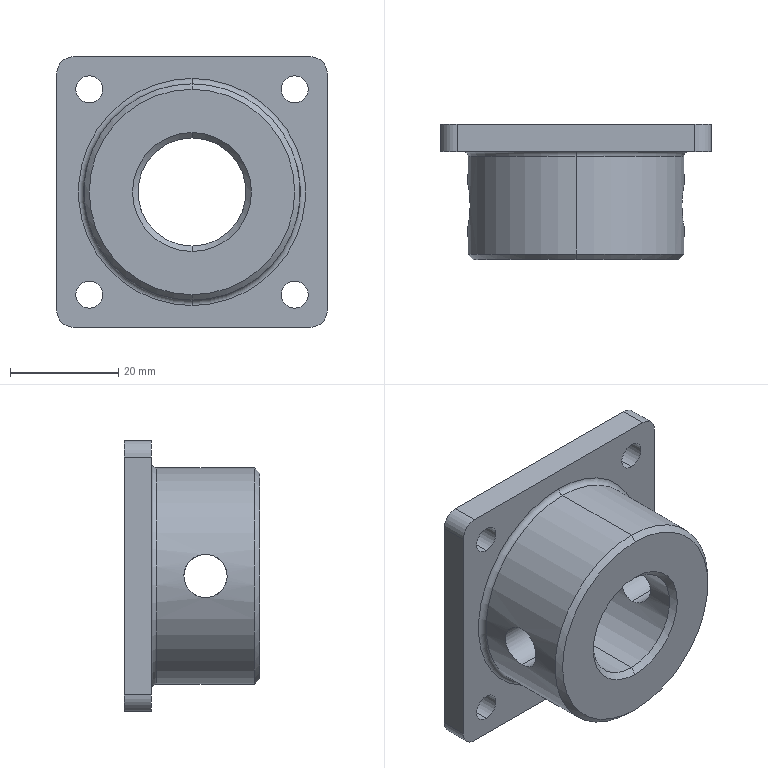Part | SolidWorks | features ICE 4, Fillet 2, Chamfer 1, Extrusion 1 | 1 solid | 33 faces | box 50 x 25 x 50 mm | volume 28265 mm3 | cylinder 20 | plane 7 | cone 4 | torus 2 | commonest cylinder face diameters 5 x8 6 x4 8 x4 20 x2 40 x2
STEP:
#1=CARTESIAN_POINT('',(0.,0.,-19.));
#2=VERTEX_POINT('',#1);
#3=CARTESIAN_POINT('',(0.,0.,19.));
#4=VERTEX_POINT('',#3);
#5=CARTESIAN_POINT('',(0.,0.,0.));
#6=DIRECTION('',(0.,-1.,0.));
#7=DIRECTION('',(0.,0.,1.));
#8=AXIS2_PLACEMENT_3D('',#5,#6,#7);
#9=CIRCLE('',#8,19.);
#10=EDGE_CURVE('',#2,#4,#9,.T.);
#11=ORIENTED_EDGE('',*,*,#10,.F.);
#12=CARTESIAN_POINT('',(0.,1.,-20.));
#13=VERTEX_POINT('',#12);
#14=CARTESIAN_POINT('',(0.,1.,-20.));
#15=DIRECTION('',(0.,0.7071,-0.7071));
#16=VECTOR('',#15,1000.);
#17=LINE('',#14,#16);
#18=EDGE_CURVE('',#2,#13,#17,.T.);
#19=ORIENTED_EDGE('',*,*,#18,.T.);
#20=CARTESIAN_POINT('',(0.,1.,20.));
#21=VERTEX_POINT('',#20);
#22=CARTESIAN_POINT('',(0.,1.,0.));
#23=DIRECTION('',(0.,1.,0.));
#24=DIRECTION('',(0.,0.,1.));
#25=AXIS2_PLACEMENT_3D('',#22,#23,#24);
#26=CIRCLE('',#25,20.);
#27=EDGE_CURVE('',#21,#13,#26,.T.);
#28=ORIENTED_EDGE('',*,*,#27,.F.);
#29=CARTESIAN_POINT('',(0.,1.,20.));
#30=DIRECTION('',(0.,0.7071,0.7071));
#31=VECTOR('',#30,1000.);
#32=LINE('',#29,#31);
#33=EDGE_CURVE('',#4,#21,#32,.T.);
#34=ORIENTED_EDGE('',*,*,#33,.F.);
#35=EDGE_LOOP('',(#11,#19,#28,#34));
#36=FACE_OUTER_BOUND('',#35,.T.);
#37=CARTESIAN_POINT('',(0.,1.,0.));
#38=DIRECTION('',(0.,1.,0.));
#39=DIRECTION('',(0.,0.,1.));
#40=AXIS2_PLACEMENT_3D('',#37,#38,#39);
#41=CONICAL_SURFACE('',#40,20.,0.7854);
#42=ADVANCED_FACE('',(#36),#41,.T.);
#43=CARTESIAN_POINT('',(0.,1.,10.));
#44=VERTEX_POINT('',#43);
#45=CARTESIAN_POINT('',(0.,1.,-10.));
#46=VERTEX_POINT('',#45);
#47=CARTESIAN_POINT('',(0.,1.,0.));
#48=DIRECTION('',(0.,-1.,0.));
#49=DIRECTION('',(0.,0.,1.));
#50=AXIS2_PLACEMENT_3D('',#47,#48,#49);
#51=CIRCLE('',#50,10.);
#52=EDGE_CURVE('',#44,#46,#51,.T.);
#53=ORIENTED_EDGE('',*,*,#52,.F.);
#54=CARTESIAN_POINT('',(0.,0.,11.));
#55=VERTEX_POINT('',#54);
#56=CARTESIAN_POINT('',(0.,0.,11.));
#57=DIRECTION('',(0.,-0.7071,0.7071));
#58=VECTOR('',#57,1000.);
#59=LINE('',#56,#58);
#60=EDGE_CURVE('',#44,#55,#59,.T.);
#61=ORIENTED_EDGE('',*,*,#60,.T.);
#62=CARTESIAN_POINT('',(0.,0.,-11.));
#63=VERTEX_POINT('',#62);
#64=CARTESIAN_POINT('',(0.,0.,0.));
#65=DIRECTION('',(0.,1.,0.));
#66=DIRECTION('',(0.,0.,1.));
#67=AXIS2_PLACEMENT_3D('',#64,#65,#66);
#68=CIRCLE('',#67,11.);
#69=EDGE_CURVE('',#63,#55,#68,.T.);
#70=ORIENTED_EDGE('',*,*,#69,.F.);
#71=CARTESIAN_POINT('',(0.,0.,-11.));
#72=DIRECTION('',(0.,-0.7071,-0.7071));
#73=VECTOR('',#72,1000.);
#74=LINE('',#71,#73);
#75=EDGE_CURVE('',#46,#63,#74,.T.);
#76=ORIENTED_EDGE('',*,*,#75,.F.);
#77=EDGE_LOOP('',(#53,#61,#70,#76));
#78=FACE_OUTER_BOUND('',#77,.T.);
#79=CARTESIAN_POINT('',(0.,0.,0.));
#80=DIRECTION('',(0.,-1.,0.));
#81=DIRECTION('',(0.,0.,-1.));
#82=AXIS2_PLACEMENT_3D('',#79,#80,#81);
#83=CONICAL_SURFACE('',#82,11.,0.7854);
#84=ADVANCED_FACE('',(#78),#83,.F.);
#85=CARTESIAN_POINT('',(0.,20.,-21.));
#86=VERTEX_POINT('',#85);
#87=CARTESIAN_POINT('',(0.,20.,21.));
#88=VERTEX_POINT('',#87);
#89=CARTESIAN_POINT('',(0.,20.,0.));
#90=DIRECTION('',(0.,1.,0.));
#91=DIRECTION('',(0.,0.,1.));
#92=AXIS2_PLACEMENT_3D('',#89,#90,#91);
#93=CIRCLE('',#92,21.);
#94=EDGE_CURVE('',#86,#88,#93,.T.);
#95=ORIENTED_EDGE('',*,*,#94,.F.);
#96=CARTESIAN_POINT('',(0.,19.,-20.));
#97=VERTEX_POINT('',#96);
#98=CARTESIAN_POINT('',(0.,19.,-21.));
#99=DIRECTION('',(1.,0.,0.));
#100=DIRECTION('',(0.,0.,-1.));
#101=AXIS2_PLACEMENT_3D('',#98,#99,#100);
#102=CIRCLE('',#101,1.);
#103=EDGE_CURVE('',#86,#97,#102,.T.);
#104=ORIENTED_EDGE('',*,*,#103,.T.);
#105=CARTESIAN_POINT('',(0.,19.,20.));
#106=VERTEX_POINT('',#105);
#107=CARTESIAN_POINT('',(0.,19.,0.));
#108=DIRECTION('',(0.,-1.,0.));
#109=DIRECTION('',(0.,0.,1.));
#110=AXIS2_PLACEMENT_3D('',#107,#108,#109);
#111=CIRCLE('',#110,20.);
#112=EDGE_CURVE('',#106,#97,#111,.T.);
#113=ORIENTED_EDGE('',*,*,#112,.F.);
#114=CARTESIAN_POINT('',(0.,19.,21.));
#115=DIRECTION('',(-1.,0.,0.));
#116=DIRECTION('',(0.,0.,1.));
#117=AXIS2_PLACEMENT_3D('',#114,#115,#116);
#118=CIRCLE('',#117,1.);
#119=EDGE_CURVE('',#88,#106,#118,.T.);
#120=ORIENTED_EDGE('',*,*,#119,.F.);
#121=EDGE_LOOP('',(#95,#104,#113,#120));
#122=FACE_OUTER_BOUND('',#121,.T.);
#123=CARTESIAN_POINT('',(0.,19.,0.));
#124=DIRECTION('',(0.,1.,0.));
#125=DIRECTION('',(0.,0.,1.));
#126=AXIS2_PLACEMENT_3D('',#123,#124,#125);
#127=TOROIDAL_SURFACE('',#126,21.,1.);
#128=ADVANCED_FACE('',(#122),#127,.F.);
#129=CARTESIAN_POINT('',(19.,20.,-21.5));
#130=VERTEX_POINT('',#129);
#131=CARTESIAN_POINT('',(19.,20.,-16.5));
#132=VERTEX_POINT('',#131);
#133=CARTESIAN_POINT('',(19.,20.,-19.));
#134=DIRECTION('',(0.,1.,0.));
#135=DIRECTION('',(0.,0.,1.));
#136=AXIS2_PLACEMENT_3D('',#133,#134,#135);
#137=CIRCLE('',#136,2.5);
#138=EDGE_CURVE('',#130,#132,#137,.T.);
#139=ORIENTED_EDGE('',*,*,#138,.F.);
#140=CARTESIAN_POINT('',(19.,25.,-21.5));
#141=VERTEX_POINT('',#140);
#142=CARTESIAN_POINT('',(19.,15.,-21.5));
#143=DIRECTION('',(0.,1.,0.));
#144=VECTOR('',#143,1000.);
#145=LINE('',#142,#144);
#146=EDGE_CURVE('',#130,#141,#145,.T.);
#147=ORIENTED_EDGE('',*,*,#146,.T.);
#148=CARTESIAN_POINT('',(19.,25.,-16.5));
#149=VERTEX_POINT('',#148);
#150=CARTESIAN_POINT('',(19.,25.,-19.));
#151=DIRECTION('',(0.,1.,0.));
#152=DIRECTION('',(0.,0.,1.));
#153=AXIS2_PLACEMENT_3D('',#150,#151,#152);
#154=CIRCLE('',#153,2.5);
#155=EDGE_CURVE('',#141,#149,#154,.T.);
#156=ORIENTED_EDGE('',*,*,#155,.T.);
#157=CARTESIAN_POINT('',(19.,15.,-16.5));
#158=DIRECTION('',(0.,1.,0.));
#159=VECTOR('',#158,1000.);
#160=LINE('',#157,#159);
#161=EDGE_CURVE('',#132,#149,#160,.T.);
#162=ORIENTED_EDGE('',*,*,#161,.F.);
#163=EDGE_LOOP('',(#139,#147,#156,#162));
#164=FACE_OUTER_BOUND('',#163,.T.);
#165=CARTESIAN_POINT('',(19.,15.,-19.));
#166=DIRECTION('',(0.,1.,0.));
#167=DIRECTION('',(0.,0.,1.));
#168=AXIS2_PLACEMENT_3D('',#165,#166,#167);
#169=CYLINDRICAL_SURFACE('',#168,2.5);
#170=ADVANCED_FACE('',(#164),#169,.F.);
#171=CARTESIAN_POINT('',(-19.,20.,16.5));
#172=VERTEX_POINT('',#171);
#173=CARTESIAN_POINT('',(-19.,20.,21.5));
#174=VERTEX_POINT('',#173);
#175=CARTESIAN_POINT('',(-19.,20.,19.));
#176=DIRECTION('',(0.,1.,0.));
#177=DIRECTION('',(0.,0.,1.));
#178=AXIS2_PLACEMENT_3D('',#175,#176,#177);
#179=CIRCLE('',#178,2.5);
#180=EDGE_CURVE('',#172,#174,#179,.T.);
#181=ORIENTED_EDGE('',*,*,#180,.F.);
#182=CARTESIAN_POINT('',(-19.,25.,16.5));
#183=VERTEX_POINT('',#182);
#184=CARTESIAN_POINT('',(-19.,15.,16.5));
#185=DIRECTION('',(0.,1.,0.));
#186=VECTOR('',#185,1000.);
#187=LINE('',#184,#186);
#188=EDGE_CURVE('',#172,#183,#187,.T.);
#189=ORIENTED_EDGE('',*,*,#188,.T.);
#190=CARTESIAN_POINT('',(-19.,25.,21.5));
#191=VERTEX_POINT('',#190);
#192=CARTESIAN_POINT('',(-19.,25.,19.));
#193=DIRECTION('',(0.,1.,0.));
#194=DIRECTION('',(0.,0.,1.));
#195=AXIS2_PLACEMENT_3D('',#192,#193,#194);
#196=CIRCLE('',#195,2.5);
#197=EDGE_CURVE('',#183,#191,#196,.T.);
#198=ORIENTED_EDGE('',*,*,#197,.T.);
#199=CARTESIAN_POINT('',(-19.,15.,21.5));
#200=DIRECTION('',(0.,1.,0.));
#201=VECTOR('',#200,1000.);
#202=LINE('',#199,#201);
#203=EDGE_CURVE('',#174,#191,#202,.T.);
#204=ORIENTED_EDGE('',*,*,#203,.F.);
#205=EDGE_LOOP('',(#181,#189,#198,#204));
#206=FACE_OUTER_BOUND('',#205,.T.);
#207=CARTESIAN_POINT('',(-19.,15.,19.));
#208=DIRECTION('',(0.,1.,0.));
#209=DIRECTION('',(0.,0.,1.));
#210=AXIS2_PLACEMENT_3D('',#207,#208,#209);
#211=CYLINDRICAL_SURFACE('',#210,2.5);
#212=ADVANCED_FACE('',(#206),#211,.F.);
#213=CARTESIAN_POINT('',(19.,20.,16.5));
#214=VERTEX_POINT('',#213);
#215=CARTESIAN_POINT('',(19.,20.,21.5));
#216=VERTEX_POINT('',#215);
#217=CARTESIAN_POINT('',(19.,20.,19.));
#218=DIRECTION('',(0.,1.,0.));
#219=DIRECTION('',(0.,0.,1.));
#220=AXIS2_PLACEMENT_3D('',#217,#218,#219);
#221=CIRCLE('',#220,2.5);
#222=EDGE_CURVE('',#214,#216,#221,.T.);
#223=ORIENTED_EDGE('',*,*,#222,.F.);
#224=CARTESIAN_POINT('',(19.,25.,16.5));
#225=VERTEX_POINT('',#224);
#226=CARTESIAN_POINT('',(19.,15.,16.5));
#227=DIRECTION('',(0.,1.,0.));
#228=VECTOR('',#227,1000.);
#229=LINE('',#226,#228);
#230=EDGE_CURVE('',#214,#225,#229,.T.);
#231=ORIENTED_EDGE('',*,*,#230,.T.);
#232=CARTESIAN_POINT('',(19.,25.,21.5));
#233=VERTEX_POINT('',#232);
#234=CARTESIAN_POINT('',(19.,25.,19.));
#235=DIRECTION('',(0.,1.,0.));
#236=DIRECTION('',(0.,0.,1.));
#237=AXIS2_PLACEMENT_3D('',#234,#235,#236);
#238=CIRCLE('',#237,2.5);
#239=EDGE_CURVE('',#225,#233,#238,.T.);
#240=ORIENTED_EDGE('',*,*,#239,.T.);
#241=CARTESIAN_POINT('',(19.,15.,21.5));
#242=DIRECTION('',(0.,1.,0.));
#243=VECTOR('',#242,1000.);
#244=LINE('',#241,#243);
#245=EDGE_CURVE('',#216,#233,#244,.T.);
#246=ORIENTED_EDGE('',*,*,#245,.F.);
#247=EDGE_LOOP('',(#223,#231,#240,#246));
#248=FACE_OUTER_BOUND('',#247,.T.);
#249=CARTESIAN_POINT('',(19.,15.,19.));
#250=DIRECTION('',(0.,1.,0.));
#251=DIRECTION('',(0.,0.,1.));
#252=AXIS2_PLACEMENT_3D('',#249,#250,#251);
#253=CYLINDRICAL_SURFACE('',#252,2.5);
#254=ADVANCED_FACE('',(#248),#253,.F.);
#255=CARTESIAN_POINT('',(-19.,20.,-21.5));
#256=VERTEX_POINT('',#255);
#257=CARTESIAN_POINT('',(-19.,20.,-16.5));
#258=VERTEX_POINT('',#257);
#259=CARTESIAN_POINT('',(-19.,20.,-19.));
#260=DIRECTION('',(0.,1.,0.));
#261=DIRECTION('',(0.,0.,1.));
#262=AXIS2_PLACEMENT_3D('',#259,#260,#261);
#263=CIRCLE('',#262,2.5);
#264=EDGE_CURVE('',#256,#258,#263,.T.);
#265=ORIENTED_EDGE('',*,*,#264,.F.);
#266=CARTESIAN_POINT('',(-19.,25.,-21.5));
#267=VERTEX_POINT('',#266);
#268=CARTESIAN_POINT('',(-19.,15.,-21.5));
#269=DIRECTION('',(0.,1.,0.));
#270=VECTOR('',#269,1000.);
#271=LINE('',#268,#270);
#272=EDGE_CURVE('',#256,#267,#271,.T.);
#273=ORIENTED_EDGE('',*,*,#272,.T.);
#274=CARTESIAN_POINT('',(-19.,25.,-16.5));
#275=VERTEX_POINT('',#274);
#276=CARTESIAN_POINT('',(-19.,25.,-19.));
#277=DIRECTION('',(0.,1.,0.));
#278=DIRECTION('',(0.,0.,1.));
#279=AXIS2_PLACEMENT_3D('',#276,#277,#278);
#280=CIRCLE('',#279,2.5);
#281=EDGE_CURVE('',#267,#275,#280,.T.);
#282=ORIENTED_EDGE('',*,*,#281,.T.);
#283=CARTESIAN_POINT('',(-19.,15.,-16.5));
#284=DIRECTION('',(0.,1.,0.));
#285=VECTOR('',#284,1000.);
#286=LINE('',#283,#285);
#287=EDGE_CURVE('',#258,#275,#286,.T.);
#288=ORIENTED_EDGE('',*,*,#287,.F.);
#289=EDGE_LOOP('',(#265,#273,#282,#288));
#290=FACE_OUTER_BOUND('',#289,.T.);
#291=CARTESIAN_POINT('',(-19.,15.,-19.));
#292=DIRECTION('',(0.,1.,0.));
#293=DIRECTION('',(0.,0.,1.));
#294=AXIS2_PLACEMENT_3D('',#291,#292,#293);
#295=CYLINDRICAL_SURFACE('',#294,2.5);
#296=ADVANCED_FACE('',(#290),#295,.F.);
#297=CARTESIAN_POINT('',(-9.165,10.,4.));
#298=VERTEX_POINT('',#297);
#299=CARTESIAN_POINT('',(-9.165,10.,-4.));
#300=VERTEX_POINT('',#299);
#301=CARTESIAN_POINT('',(-9.165,10.,4.));
#302=CARTESIAN_POINT('',(-9.165,10.267,4.));
#303=CARTESIAN_POINT('',(-9.177,10.53,3.973));
#304=CARTESIAN_POINT('',(-9.221,11.045,3.87));
#305=CARTESIAN_POINT('',(-9.254,11.3,3.792));
#306=CARTESIAN_POINT('',(-9.334,11.783,3.59));
#307=CARTESIAN_POINT('',(-9.381,12.011,3.467));
#308=CARTESIAN_POINT('',(-9.483,12.444,3.177));
#309=CARTESIAN_POINT('',(-9.538,12.646,3.011));
#310=CARTESIAN_POINT('',(-9.646,13.011,2.646));
#311=CARTESIAN_POINT('',(-9.699,13.176,2.445));
#312=CARTESIAN_POINT('',(-9.798,13.468,2.01));
#313=CARTESIAN_POINT('',(-9.843,13.591,1.781));
#314=CARTESIAN_POINT('',(-9.918,13.792,1.301));
#315=CARTESIAN_POINT('',(-9.949,13.87,1.046));
#316=CARTESIAN_POINT('',(-9.989,13.974,0.5279));
#317=CARTESIAN_POINT('',(-10.,14.,0.2663));
#318=CARTESIAN_POINT('',(-10.,14.,-0.2622));
#319=CARTESIAN_POINT('',(-9.989,13.973,-0.5302));
#320=CARTESIAN_POINT('',(-9.949,13.87,-1.046));
#321=CARTESIAN_POINT('',(-9.919,13.793,-1.297));
#322=CARTESIAN_POINT('',(-9.842,13.589,-1.785));
#323=CARTESIAN_POINT('',(-9.798,13.466,-2.014));
#324=CARTESIAN_POINT('',(-9.699,13.176,-2.445));
#325=CARTESIAN_POINT('',(-9.645,13.009,-2.648));
#326=CARTESIAN_POINT('',(-9.537,12.642,-3.014));
#327=CARTESIAN_POINT('',(-9.483,12.443,-3.178));
#328=CARTESIAN_POINT('',(-9.381,12.011,-3.467));
#329=CARTESIAN_POINT('',(-9.333,11.778,-3.592));
#330=CARTESIAN_POINT('',(-9.254,11.298,-3.792));
#331=CARTESIAN_POINT('',(-9.221,11.048,-3.869));
#332=CARTESIAN_POINT('',(-9.177,10.527,-3.974));
#333=CARTESIAN_POINT('',(-9.165,10.263,-4.));
#334=CARTESIAN_POINT('',(-9.165,10.,-4.));
#335=B_SPLINE_CURVE_WITH_KNOTS('',3,(#301,#302,#303,#304,#305,#306,#307,#308,#309,#310,#311,#312,#313,#314,#315,#316,#317,#318,#319,#320,#321,#322,#323,#324,#325,#326,#327,#328,#329,#330,#331,#332,#333,#334),.UNSPECIFIED.,.F.,.F.,(4,2,2,2,2,2,2,2,2,2,2,2,2,2,2,2,4),(0.,0.0007899,0.00158,0.00237,0.00316,0.00395,0.00474,0.00553,0.006319,0.007109,0.007899,0.008689,0.009479,0.01027,0.01106,0.01185,0.01264),.UNSPECIFIED.);
#336=EDGE_CURVE('',#298,#300,#335,.T.);
#337=ORIENTED_EDGE('',*,*,#336,.T.);
#338=CARTESIAN_POINT('',(-9.165,10.,-4.));
#339=CARTESIAN_POINT('',(-9.165,9.737,-4.));
#340=CARTESIAN_POINT('',(-9.177,9.471,-3.974));
#341=CARTESIAN_POINT('',(-9.221,8.952,-3.869));
#342=CARTESIAN_POINT('',(-9.254,8.702,-3.793));
#343=CARTESIAN_POINT('',(-9.334,8.219,-3.591));
#344=CARTESIAN_POINT('',(-9.381,7.987,-3.466));
#345=CARTESIAN_POINT('',(-9.483,7.557,-3.178));
#346=CARTESIAN_POINT('',(-9.537,7.356,-3.013));
#347=CARTESIAN_POINT('',(-9.646,6.987,-2.644));
#348=CARTESIAN_POINT('',(-9.699,6.823,-2.444));
#349=CARTESIAN_POINT('',(-9.797,6.535,-2.015));
#350=CARTESIAN_POINT('',(-9.843,6.409,-1.782));
#351=CARTESIAN_POINT('',(-9.918,6.208,-1.299));
#352=CARTESIAN_POINT('',(-9.948,6.131,-1.049));
#353=CARTESIAN_POINT('',(-9.989,6.027,-0.5334));
#354=CARTESIAN_POINT('',(-10.,6.,-0.2654));
#355=CARTESIAN_POINT('',(-10.,6.,0.2618));
#356=CARTESIAN_POINT('',(-9.99,6.026,0.5238));
#357=CARTESIAN_POINT('',(-9.949,6.13,1.045));
#358=CARTESIAN_POINT('',(-9.919,6.207,1.297));
#359=CARTESIAN_POINT('',(-9.843,6.408,1.779));
#360=CARTESIAN_POINT('',(-9.798,6.533,2.012));
#361=CARTESIAN_POINT('',(-9.699,6.823,2.444));
#362=CARTESIAN_POINT('',(-9.646,6.987,2.644));
#363=CARTESIAN_POINT('',(-9.538,7.354,3.011));
#364=CARTESIAN_POINT('',(-9.483,7.557,3.177));
#365=CARTESIAN_POINT('',(-9.382,7.986,3.465));
#366=CARTESIAN_POINT('',(-9.335,8.214,3.589));
#367=CARTESIAN_POINT('',(-9.254,8.7,3.792));
#368=CARTESIAN_POINT('',(-9.221,8.952,3.869));
#369=CARTESIAN_POINT('',(-9.177,9.467,3.973));
#370=CARTESIAN_POINT('',(-9.165,9.733,4.));
#371=CARTESIAN_POINT('',(-9.165,10.,4.));
#372=B_SPLINE_CURVE_WITH_KNOTS('',3,(#338,#339,#340,#341,#342,#343,#344,#345,#346,#347,#348,#349,#350,#351,#352,#353,#354,#355,#356,#357,#358,#359,#360,#361,#362,#363,#364,#365,#366,#367,#368,#369,#370,#371),.UNSPECIFIED.,.F.,.F.,(4,2,2,2,2,2,2,2,2,2,2,2,2,2,2,2,4),(0.01264,0.01343,0.01422,0.01501,0.0158,0.01658,0.01737,0.01816,0.01895,0.01974,0.02053,0.02132,0.02211,0.0229,0.02369,0.02448,0.02527),.UNSPECIFIED.);
#373=EDGE_CURVE('',#300,#298,#372,.T.);
#374=ORIENTED_EDGE('',*,*,#373,.T.);
#375=EDGE_LOOP('',(#337,#374));
#376=FACE_BOUND('',#375,.T.);
#377=ORIENTED_EDGE('',*,*,#52,.T.);
#378=CARTESIAN_POINT('',(0.,25.,-10.));
#379=VERTEX_POINT('',#378);
#380=CARTESIAN_POINT('',(0.,0.,-10.));
#381=DIRECTION('',(0.,1.,0.));
#382=VECTOR('',#381,1000.);
#383=LINE('',#380,#382);
#384=EDGE_CURVE('',#46,#379,#383,.T.);
#385=ORIENTED_EDGE('',*,*,#384,.T.);
#386=CARTESIAN_POINT('',(0.,25.,10.));
#387=VERTEX_POINT('',#386);
#388=CARTESIAN_POINT('',(0.,25.,0.));
#389=DIRECTION('',(0.,1.,0.));
#390=DIRECTION('',(0.,0.,1.));
#391=AXIS2_PLACEMENT_3D('',#388,#389,#390);
#392=CIRCLE('',#391,10.);
#393=EDGE_CURVE('',#379,#387,#392,.T.);
#394=ORIENTED_EDGE('',*,*,#393,.T.);
#395=CARTESIAN_POINT('',(0.,0.,10.));
#396=DIRECTION('',(0.,1.,0.));
#397=VECTOR('',#396,1000.);
#398=LINE('',#395,#397);
#399=EDGE_CURVE('',#44,#387,#398,.T.);
#400=ORIENTED_EDGE('',*,*,#399,.F.);
#401=EDGE_LOOP('',(#377,#385,#394,#400));
#402=FACE_OUTER_BOUND('',#401,.T.);
#403=CARTESIAN_POINT('',(0.,0.,0.));
#404=DIRECTION('',(0.,1.,0.));
#405=DIRECTION('',(0.,0.,1.));
#406=AXIS2_PLACEMENT_3D('',#403,#404,#405);
#407=CYLINDRICAL_SURFACE('',#406,10.);
#408=ADVANCED_FACE('',(#376,#402),#407,.F.);
#409=ORIENTED_EDGE('',*,*,#373,.F.);
#410=CARTESIAN_POINT('',(-19.596,10.,-4.));
#411=VERTEX_POINT('',#410);
#412=CARTESIAN_POINT('',(25.,10.,-4.));
#413=DIRECTION('',(-1.,0.,0.));
#414=VECTOR('',#413,1000.);
#415=LINE('',#412,#414);
#416=EDGE_CURVE('',#300,#411,#415,.T.);
#417=ORIENTED_EDGE('',*,*,#416,.T.);
#418=CARTESIAN_POINT('',(-19.596,10.,4.));
#419=VERTEX_POINT('',#418);
#420=CARTESIAN_POINT('',(-19.596,10.,-4.));
#421=CARTESIAN_POINT('',(-19.596,9.739,-4.));
#422=CARTESIAN_POINT('',(-19.601,9.478,-3.975));
#423=CARTESIAN_POINT('',(-19.622,8.96,-3.872));
#424=CARTESIAN_POINT('',(-19.637,8.709,-3.795));
#425=CARTESIAN_POINT('',(-19.674,8.227,-3.595));
#426=CARTESIAN_POINT('',(-19.697,7.994,-3.47));
#427=CARTESIAN_POINT('',(-19.746,7.559,-3.179));
#428=CARTESIAN_POINT('',(-19.772,7.358,-3.014));
#429=CARTESIAN_POINT('',(-19.825,6.989,-2.646));
#430=CARTESIAN_POINT('',(-19.852,6.82,-2.441));
#431=CARTESIAN_POINT('',(-19.9,6.531,-2.008));
#432=CARTESIAN_POINT('',(-19.922,6.407,-1.778));
#433=CARTESIAN_POINT('',(-19.96,6.206,-1.293));
#434=CARTESIAN_POINT('',(-19.975,6.129,-1.04));
#435=CARTESIAN_POINT('',(-19.995,6.026,-0.5284));
#436=CARTESIAN_POINT('',(-20.,6.,-0.2661));
#437=CARTESIAN_POINT('',(-20.,6.,0.2621));
#438=CARTESIAN_POINT('',(-19.995,6.026,0.5222));
#439=CARTESIAN_POINT('',(-19.975,6.127,1.035));
#440=CARTESIAN_POINT('',(-19.96,6.205,1.29));
#441=CARTESIAN_POINT('',(-19.923,6.405,1.773));
#442=CARTESIAN_POINT('',(-19.901,6.528,2.003));
#443=CARTESIAN_POINT('',(-19.852,6.818,2.438));
#444=CARTESIAN_POINT('',(-19.825,6.986,2.643));
#445=CARTESIAN_POINT('',(-19.773,7.354,3.011));
#446=CARTESIAN_POINT('',(-19.747,7.555,3.177));
#447=CARTESIAN_POINT('',(-19.697,7.993,3.47));
#448=CARTESIAN_POINT('',(-19.675,8.223,3.593));
#449=CARTESIAN_POINT('',(-19.637,8.704,3.793));
#450=CARTESIAN_POINT('',(-19.622,8.957,3.871));
#451=CARTESIAN_POINT('',(-19.601,9.474,3.974));
#452=CARTESIAN_POINT('',(-19.596,9.735,4.));
#453=CARTESIAN_POINT('',(-19.596,10.,4.));
#454=B_SPLINE_CURVE_WITH_KNOTS('',3,(#420,#421,#422,#423,#424,#425,#426,#427,#428,#429,#430,#431,#432,#433,#434,#435,#436,#437,#438,#439,#440,#441,#442,#443,#444,#445,#446,#447,#448,#449,#450,#451,#452,#453),.UNSPECIFIED.,.F.,.F.,(4,2,2,2,2,2,2,2,2,2,2,2,2,2,2,2,4),(0.01254,0.01332,0.0141,0.01489,0.01567,0.01645,0.01724,0.01802,0.0188,0.01959,0.02037,0.02115,0.02194,0.02272,0.0235,0.02429,0.02507),.UNSPECIFIED.);
#455=EDGE_CURVE('',#411,#419,#454,.T.);
#456=ORIENTED_EDGE('',*,*,#455,.T.);
#457=CARTESIAN_POINT('',(25.,10.,4.));
#458=DIRECTION('',(-1.,0.,0.));
#459=VECTOR('',#458,1000.);
#460=LINE('',#457,#459);
#461=EDGE_CURVE('',#298,#419,#460,.T.);
#462=ORIENTED_EDGE('',*,*,#461,.F.);
#463=EDGE_LOOP('',(#409,#417,#456,#462));
#464=FACE_OUTER_BOUND('',#463,.T.);
#465=CARTESIAN_POINT('',(25.,10.,0.));
#466=DIRECTION('',(-1.,0.,0.));
#467=DIRECTION('',(0.,0.,1.));
#468=AXIS2_PLACEMENT_3D('',#465,#466,#467);
#469=CYLINDRICAL_SURFACE('',#468,4.);
#470=ADVANCED_FACE('',(#464),#469,.F.);
#471=CARTESIAN_POINT('',(19.596,10.,4.));
#472=VERTEX_POINT('',#471);
#473=CARTESIAN_POINT('',(19.596,10.,-4.));
#474=VERTEX_POINT('',#473);
#475=CARTESIAN_POINT('',(19.596,10.,4.));
#476=CARTESIAN_POINT('',(19.596,9.735,4.));
#477=CARTESIAN_POINT('',(19.601,9.475,3.974));
#478=CARTESIAN_POINT('',(19.622,8.962,3.872));
#479=CARTESIAN_POINT('',(19.637,8.708,3.795));
#480=CARTESIAN_POINT('',(19.675,8.224,3.594));
#481=CARTESIAN_POINT('',(19.697,7.994,3.471));
#482=CARTESIAN_POINT('',(19.746,7.56,3.18));
#483=CARTESIAN_POINT('',(19.773,7.355,3.012));
#484=CARTESIAN_POINT('',(19.825,6.987,2.644));
#485=CARTESIAN_POINT('',(19.851,6.822,2.443));
#486=CARTESIAN_POINT('',(19.9,6.529,2.006));
#487=CARTESIAN_POINT('',(19.923,6.405,1.774));
#488=CARTESIAN_POINT('',(19.96,6.206,1.293));
#489=CARTESIAN_POINT('',(19.975,6.129,1.04));
#490=CARTESIAN_POINT('',(19.995,6.026,0.5232));
#491=CARTESIAN_POINT('',(20.,6.,0.2632));
#492=CARTESIAN_POINT('',(20.,6.,-0.2601));
#493=CARTESIAN_POINT('',(19.995,6.026,-0.5259));
#494=CARTESIAN_POINT('',(19.975,6.129,-1.039));
#495=CARTESIAN_POINT('',(19.96,6.204,-1.289));
#496=CARTESIAN_POINT('',(19.923,6.405,-1.774));
#497=CARTESIAN_POINT('',(19.9,6.53,-2.007));
#498=CARTESIAN_POINT('',(19.852,6.82,-2.44));
#499=CARTESIAN_POINT('',(19.826,6.986,-2.643));
#500=CARTESIAN_POINT('',(19.772,7.358,-3.015));
#501=CARTESIAN_POINT('',(19.746,7.559,-3.18));
#502=CARTESIAN_POINT('',(19.697,7.992,-3.469));
#503=CARTESIAN_POINT('',(19.675,8.226,-3.595));
#504=CARTESIAN_POINT('',(19.637,8.71,-3.795));
#505=CARTESIAN_POINT('',(19.622,8.959,-3.871));
#506=CARTESIAN_POINT('',(19.601,9.473,-3.974));
#507=CARTESIAN_POINT('',(19.596,9.739,-4.));
#508=CARTESIAN_POINT('',(19.596,10.,-4.));
#509=B_SPLINE_CURVE_WITH_KNOTS('',3,(#475,#476,#477,#478,#479,#480,#481,#482,#483,#484,#485,#486,#487,#488,#489,#490,#491,#492,#493,#494,#495,#496,#497,#498,#499,#500,#501,#502,#503,#504,#505,#506,#507,#508),.UNSPECIFIED.,.F.,.F.,(4,2,2,2,2,2,2,2,2,2,2,2,2,2,2,2,4),(0.,0.0007836,0.001567,0.002351,0.003134,0.003918,0.004702,0.005485,0.006269,0.007052,0.007836,0.008619,0.009403,0.01019,0.01097,0.01175,0.01254),.UNSPECIFIED.);
#510=EDGE_CURVE('',#472,#474,#509,.T.);
#511=ORIENTED_EDGE('',*,*,#510,.F.);
#512=CARTESIAN_POINT('',(19.596,10.,-4.));
#513=CARTESIAN_POINT('',(19.596,10.261,-4.));
#514=CARTESIAN_POINT('',(19.601,10.522,-3.975));
#515=CARTESIAN_POINT('',(19.622,11.04,-3.872));
#516=CARTESIAN_POINT('',(19.637,11.291,-3.795));
#517=CARTESIAN_POINT('',(19.674,11.773,-3.595));
#518=CARTESIAN_POINT('',(19.697,12.006,-3.47));
#519=CARTESIAN_POINT('',(19.746,12.441,-3.179));
#520=CARTESIAN_POINT('',(19.772,12.642,-3.014));
#521=CARTESIAN_POINT('',(19.825,13.011,-2.646));
#522=CARTESIAN_POINT('',(19.852,13.18,-2.441));
#523=CARTESIAN_POINT('',(19.9,13.469,-2.008));
#524=CARTESIAN_POINT('',(19.922,13.593,-1.778));
#525=CARTESIAN_POINT('',(19.96,13.794,-1.293));
#526=CARTESIAN_POINT('',(19.975,13.871,-1.04));
#527=CARTESIAN_POINT('',(19.995,13.974,-0.5284));
#528=CARTESIAN_POINT('',(20.,14.,-0.2661));
#529=CARTESIAN_POINT('',(20.,14.,0.2621));
#530=CARTESIAN_POINT('',(19.995,13.974,0.5222));
#531=CARTESIAN_POINT('',(19.975,13.873,1.035));
#532=CARTESIAN_POINT('',(19.96,13.795,1.29));
#533=CARTESIAN_POINT('',(19.923,13.595,1.773));
#534=CARTESIAN_POINT('',(19.901,13.472,2.003));
#535=CARTESIAN_POINT('',(19.852,13.182,2.438));
#536=CARTESIAN_POINT('',(19.825,13.014,2.643));
#537=CARTESIAN_POINT('',(19.773,12.646,3.011));
#538=CARTESIAN_POINT('',(19.747,12.445,3.177));
#539=CARTESIAN_POINT('',(19.697,12.007,3.47));
#540=CARTESIAN_POINT('',(19.675,11.777,3.593));
#541=CARTESIAN_POINT('',(19.637,11.296,3.793));
#542=CARTESIAN_POINT('',(19.622,11.043,3.871));
#543=CARTESIAN_POINT('',(19.601,10.526,3.974));
#544=CARTESIAN_POINT('',(19.596,10.265,4.));
#545=CARTESIAN_POINT('',(19.596,10.,4.));
#546=B_SPLINE_CURVE_WITH_KNOTS('',3,(#512,#513,#514,#515,#516,#517,#518,#519,#520,#521,#522,#523,#524,#525,#526,#527,#528,#529,#530,#531,#532,#533,#534,#535,#536,#537,#538,#539,#540,#541,#542,#543,#544,#545),.UNSPECIFIED.,.F.,.F.,(4,2,2,2,2,2,2,2,2,2,2,2,2,2,2,2,4),(0.01254,0.01332,0.0141,0.01489,0.01567,0.01645,0.01724,0.01802,0.0188,0.01959,0.02037,0.02115,0.02194,0.02272,0.0235,0.02429,0.02507),.UNSPECIFIED.);
#547=EDGE_CURVE('',#474,#472,#546,.T.);
#548=ORIENTED_EDGE('',*,*,#547,.F.);
#549=EDGE_LOOP('',(#511,#548));
#550=FACE_BOUND('',#549,.T.);
#551=CARTESIAN_POINT('',(0.,19.,0.));
#552=DIRECTION('',(0.,-1.,0.));
#553=DIRECTION('',(0.,0.,1.));
#554=AXIS2_PLACEMENT_3D('',#551,#552,#553);
#555=CIRCLE('',#554,20.);
#556=EDGE_CURVE('',#97,#106,#555,.T.);
#557=ORIENTED_EDGE('',*,*,#556,.T.);
#558=CARTESIAN_POINT('',(0.,20.,20.));
#559=DIRECTION('',(0.,-1.,0.));
#560=VECTOR('',#559,1000.);
#561=LINE('',#558,#560);
#562=EDGE_CURVE('',#106,#21,#561,.T.);
#563=ORIENTED_EDGE('',*,*,#562,.T.);
#564=ORIENTED_EDGE('',*,*,#27,.T.);
#565=CARTESIAN_POINT('',(0.,20.,-20.));
#566=DIRECTION('',(0.,-1.,0.));
#567=VECTOR('',#566,1000.);
#568=LINE('',#565,#567);
#569=EDGE_CURVE('',#97,#13,#568,.T.);
#570=ORIENTED_EDGE('',*,*,#569,.F.);
#571=EDGE_LOOP('',(#557,#563,#564,#570));
#572=FACE_OUTER_BOUND('',#571,.T.);
#573=CARTESIAN_POINT('',(0.,20.,0.));
#574=DIRECTION('',(0.,-1.,0.));
#575=DIRECTION('',(0.,0.,-1.));
#576=AXIS2_PLACEMENT_3D('',#573,#574,#575);
#577=CYLINDRICAL_SURFACE('',#576,20.);
#578=ADVANCED_FACE('',(#550,#572),#577,.T.);
#579=ORIENTED_EDGE('',*,*,#510,.T.);
#580=CARTESIAN_POINT('',(9.165,10.,-4.));
#581=VERTEX_POINT('',#580);
#582=CARTESIAN_POINT('',(25.,10.,-4.));
#583=DIRECTION('',(-1.,0.,0.));
#584=VECTOR('',#583,1000.);
#585=LINE('',#582,#584);
#586=EDGE_CURVE('',#474,#581,#585,.T.);
#587=ORIENTED_EDGE('',*,*,#586,.T.);
#588=CARTESIAN_POINT('',(9.165,10.,4.));
#589=VERTEX_POINT('',#588);
#590=CARTESIAN_POINT('',(9.165,10.,4.));
#591=CARTESIAN_POINT('',(9.165,9.733,4.));
#592=CARTESIAN_POINT('',(9.177,9.47,3.973));
#593=CARTESIAN_POINT('',(9.221,8.955,3.87));
#594=CARTESIAN_POINT('',(9.254,8.7,3.792));
#595=CARTESIAN_POINT('',(9.334,8.217,3.59));
#596=CARTESIAN_POINT('',(9.381,7.989,3.467));
#597=CARTESIAN_POINT('',(9.483,7.556,3.177));
#598=CARTESIAN_POINT('',(9.538,7.354,3.011));
#599=CARTESIAN_POINT('',(9.646,6.989,2.646));
#600=CARTESIAN_POINT('',(9.699,6.824,2.445));
#601=CARTESIAN_POINT('',(9.798,6.532,2.01));
#602=CARTESIAN_POINT('',(9.843,6.409,1.781));
#603=CARTESIAN_POINT('',(9.918,6.208,1.301));
#604=CARTESIAN_POINT('',(9.949,6.13,1.046));
#605=CARTESIAN_POINT('',(9.989,6.026,0.5279));
#606=CARTESIAN_POINT('',(10.,6.,0.2663));
#607=CARTESIAN_POINT('',(10.,6.,-0.2622));
#608=CARTESIAN_POINT('',(9.989,6.027,-0.5302));
#609=CARTESIAN_POINT('',(9.949,6.13,-1.046));
#610=CARTESIAN_POINT('',(9.919,6.207,-1.297));
#611=CARTESIAN_POINT('',(9.842,6.411,-1.785));
#612=CARTESIAN_POINT('',(9.798,6.534,-2.014));
#613=CARTESIAN_POINT('',(9.699,6.824,-2.445));
#614=CARTESIAN_POINT('',(9.645,6.991,-2.648));
#615=CARTESIAN_POINT('',(9.537,7.358,-3.014));
#616=CARTESIAN_POINT('',(9.483,7.557,-3.178));
#617=CARTESIAN_POINT('',(9.381,7.989,-3.467));
#618=CARTESIAN_POINT('',(9.333,8.222,-3.592));
#619=CARTESIAN_POINT('',(9.254,8.702,-3.792));
#620=CARTESIAN_POINT('',(9.221,8.952,-3.869));
#621=CARTESIAN_POINT('',(9.177,9.473,-3.974));
#622=CARTESIAN_POINT('',(9.165,9.737,-4.));
#623=CARTESIAN_POINT('',(9.165,10.,-4.));
#624=B_SPLINE_CURVE_WITH_KNOTS('',3,(#590,#591,#592,#593,#594,#595,#596,#597,#598,#599,#600,#601,#602,#603,#604,#605,#606,#607,#608,#609,#610,#611,#612,#613,#614,#615,#616,#617,#618,#619,#620,#621,#622,#623),.UNSPECIFIED.,.F.,.F.,(4,2,2,2,2,2,2,2,2,2,2,2,2,2,2,2,4),(0.,0.0007899,0.00158,0.00237,0.00316,0.00395,0.00474,0.00553,0.006319,0.007109,0.007899,0.008689,0.009479,0.01027,0.01106,0.01185,0.01264),.UNSPECIFIED.);
#625=EDGE_CURVE('',#589,#581,#624,.T.);
#626=ORIENTED_EDGE('',*,*,#625,.F.);
#627=CARTESIAN_POINT('',(25.,10.,4.));
#628=DIRECTION('',(-1.,0.,0.));
#629=VECTOR('',#628,1000.);
#630=LINE('',#627,#629);
#631=EDGE_CURVE('',#472,#589,#630,.T.);
#632=ORIENTED_EDGE('',*,*,#631,.F.);
#633=EDGE_LOOP('',(#579,#587,#626,#632));
#634=FACE_OUTER_BOUND('',#633,.T.);
#635=CARTESIAN_POINT('',(25.,10.,0.));
#636=DIRECTION('',(-1.,0.,0.));
#637=DIRECTION('',(0.,0.,1.));
#638=AXIS2_PLACEMENT_3D('',#635,#636,#637);
#639=CYLINDRICAL_SURFACE('',#638,4.);
#640=ADVANCED_FACE('',(#634),#639,.F.);
#641=ORIENTED_EDGE('',*,*,#586,.F.);
#642=ORIENTED_EDGE('',*,*,#547,.T.);
#643=ORIENTED_EDGE('',*,*,#631,.T.);
#644=CARTESIAN_POINT('',(9.165,10.,-4.));
#645=CARTESIAN_POINT('',(9.165,10.263,-4.));
#646=CARTESIAN_POINT('',(9.177,10.529,-3.974));
#647=CARTESIAN_POINT('',(9.221,11.048,-3.869));
#648=CARTESIAN_POINT('',(9.254,11.298,-3.793));
#649=CARTESIAN_POINT('',(9.334,11.781,-3.591));
#650=CARTESIAN_POINT('',(9.381,12.013,-3.466));
#651=CARTESIAN_POINT('',(9.483,12.443,-3.178));
#652=CARTESIAN_POINT('',(9.537,12.644,-3.013));
#653=CARTESIAN_POINT('',(9.646,13.013,-2.644));
#654=CARTESIAN_POINT('',(9.699,13.177,-2.444));
#655=CARTESIAN_POINT('',(9.797,13.465,-2.015));
#656=CARTESIAN_POINT('',(9.843,13.591,-1.782));
#657=CARTESIAN_POINT('',(9.918,13.792,-1.299));
#658=CARTESIAN_POINT('',(9.948,13.869,-1.049));
#659=CARTESIAN_POINT('',(9.989,13.973,-0.5334));
#660=CARTESIAN_POINT('',(10.,14.,-0.2654));
#661=CARTESIAN_POINT('',(10.,14.,0.2618));
#662=CARTESIAN_POINT('',(9.99,13.974,0.5238));
#663=CARTESIAN_POINT('',(9.949,13.87,1.045));
#664=CARTESIAN_POINT('',(9.919,13.793,1.297));
#665=CARTESIAN_POINT('',(9.843,13.592,1.779));
#666=CARTESIAN_POINT('',(9.798,13.467,2.012));
#667=CARTESIAN_POINT('',(9.699,13.177,2.444));
#668=CARTESIAN_POINT('',(9.646,13.013,2.644));
#669=CARTESIAN_POINT('',(9.538,12.646,3.011));
#670=CARTESIAN_POINT('',(9.483,12.443,3.177));
#671=CARTESIAN_POINT('',(9.382,12.014,3.465));
#672=CARTESIAN_POINT('',(9.335,11.786,3.589));
#673=CARTESIAN_POINT('',(9.254,11.3,3.792));
#674=CARTESIAN_POINT('',(9.221,11.048,3.869));
#675=CARTESIAN_POINT('',(9.177,10.533,3.973));
#676=CARTESIAN_POINT('',(9.165,10.267,4.));
#677=CARTESIAN_POINT('',(9.165,10.,4.));
#678=B_SPLINE_CURVE_WITH_KNOTS('',3,(#644,#645,#646,#647,#648,#649,#650,#651,#652,#653,#654,#655,#656,#657,#658,#659,#660,#661,#662,#663,#664,#665,#666,#667,#668,#669,#670,#671,#672,#673,#674,#675,#676,#677),.UNSPECIFIED.,.F.,.F.,(4,2,2,2,2,2,2,2,2,2,2,2,2,2,2,2,4),(0.01264,0.01343,0.01422,0.01501,0.0158,0.01658,0.01737,0.01816,0.01895,0.01974,0.02053,0.02132,0.02211,0.0229,0.02369,0.02448,0.02527),.UNSPECIFIED.);
#679=EDGE_CURVE('',#581,#589,#678,.T.);
#680=ORIENTED_EDGE('',*,*,#679,.F.);
#681=EDGE_LOOP('',(#641,#642,#643,#680));
#682=FACE_OUTER_BOUND('',#681,.T.);
#683=CARTESIAN_POINT('',(25.,10.,0.));
#684=DIRECTION('',(-1.,0.,0.));
#685=DIRECTION('',(0.,0.,1.));
#686=AXIS2_PLACEMENT_3D('',#683,#684,#685);
#687=CYLINDRICAL_SURFACE('',#686,4.);
#688=ADVANCED_FACE('',(#682),#687,.F.);
#689=ORIENTED_EDGE('',*,*,#562,.F.);
#690=ORIENTED_EDGE('',*,*,#112,.T.);
#691=ORIENTED_EDGE('',*,*,#569,.T.);
#692=CARTESIAN_POINT('',(0.,1.,0.));
#693=DIRECTION('',(0.,1.,0.));
#694=DIRECTION('',(0.,0.,1.));
#695=AXIS2_PLACEMENT_3D('',#692,#693,#694);
#696=CIRCLE('',#695,20.);
#697=EDGE_CURVE('',#13,#21,#696,.T.);
#698=ORIENTED_EDGE('',*,*,#697,.T.);
#699=EDGE_LOOP('',(#689,#690,#691,#698));
#700=FACE_OUTER_BOUND('',#699,.T.);
#701=CARTESIAN_POINT('',(-19.596,10.,4.));
#702=CARTESIAN_POINT('',(-19.596,10.265,4.));
#703=CARTESIAN_POINT('',(-19.601,10.525,3.974));
#704=CARTESIAN_POINT('',(-19.622,11.038,3.872));
#705=CARTESIAN_POINT('',(-19.637,11.292,3.795));
#706=CARTESIAN_POINT('',(-19.675,11.776,3.594));
#707=CARTESIAN_POINT('',(-19.697,12.006,3.471));
#708=CARTESIAN_POINT('',(-19.746,12.44,3.18));
#709=CARTESIAN_POINT('',(-19.773,12.645,3.012));
#710=CARTESIAN_POINT('',(-19.825,13.013,2.644));
#711=CARTESIAN_POINT('',(-19.851,13.178,2.443));
#712=CARTESIAN_POINT('',(-19.9,13.471,2.006));
#713=CARTESIAN_POINT('',(-19.923,13.595,1.774));
#714=CARTESIAN_POINT('',(-19.96,13.794,1.293));
#715=CARTESIAN_POINT('',(-19.975,13.871,1.04));
#716=CARTESIAN_POINT('',(-19.995,13.974,0.5232));
#717=CARTESIAN_POINT('',(-20.,14.,0.2632));
#718=CARTESIAN_POINT('',(-20.,14.,-0.2601));
#719=CARTESIAN_POINT('',(-19.995,13.974,-0.5259));
#720=CARTESIAN_POINT('',(-19.975,13.871,-1.039));
#721=CARTESIAN_POINT('',(-19.96,13.796,-1.289));
#722=CARTESIAN_POINT('',(-19.923,13.595,-1.774));
#723=CARTESIAN_POINT('',(-19.9,13.47,-2.007));
#724=CARTESIAN_POINT('',(-19.852,13.18,-2.44));
#725=CARTESIAN_POINT('',(-19.826,13.014,-2.643));
#726=CARTESIAN_POINT('',(-19.772,12.642,-3.015));
#727=CARTESIAN_POINT('',(-19.746,12.441,-3.18));
#728=CARTESIAN_POINT('',(-19.697,12.008,-3.469));
#729=CARTESIAN_POINT('',(-19.675,11.774,-3.595));
#730=CARTESIAN_POINT('',(-19.637,11.29,-3.795));
#731=CARTESIAN_POINT('',(-19.622,11.041,-3.871));
#732=CARTESIAN_POINT('',(-19.601,10.527,-3.974));
#733=CARTESIAN_POINT('',(-19.596,10.261,-4.));
#734=CARTESIAN_POINT('',(-19.596,10.,-4.));
#735=B_SPLINE_CURVE_WITH_KNOTS('',3,(#701,#702,#703,#704,#705,#706,#707,#708,#709,#710,#711,#712,#713,#714,#715,#716,#717,#718,#719,#720,#721,#722,#723,#724,#725,#726,#727,#728,#729,#730,#731,#732,#733,#734),.UNSPECIFIED.,.F.,.F.,(4,2,2,2,2,2,2,2,2,2,2,2,2,2,2,2,4),(0.,0.0007836,0.001567,0.002351,0.003134,0.003918,0.004702,0.005485,0.006269,0.007052,0.007836,0.008619,0.009403,0.01019,0.01097,0.01175,0.01254),.UNSPECIFIED.);
#736=EDGE_CURVE('',#419,#411,#735,.T.);
#737=ORIENTED_EDGE('',*,*,#736,.F.);
#738=ORIENTED_EDGE('',*,*,#455,.F.);
#739=EDGE_LOOP('',(#737,#738));
#740=FACE_BOUND('',#739,.T.);
#741=CARTESIAN_POINT('',(0.,20.,0.));
#742=DIRECTION('',(0.,-1.,0.));
#743=DIRECTION('',(0.,0.,-1.));
#744=AXIS2_PLACEMENT_3D('',#741,#742,#743);
#745=CYLINDRICAL_SURFACE('',#744,20.);
#746=ADVANCED_FACE('',(#700,#740),#745,.T.);
#747=ORIENTED_EDGE('',*,*,#69,.T.);
#748=CARTESIAN_POINT('',(0.,0.,0.));
#749=DIRECTION('',(0.,1.,0.));
#750=DIRECTION('',(0.,0.,1.));
#751=AXIS2_PLACEMENT_3D('',#748,#749,#750);
#752=CIRCLE('',#751,11.);
#753=EDGE_CURVE('',#55,#63,#752,.T.);
#754=ORIENTED_EDGE('',*,*,#753,.T.);
#755=EDGE_LOOP('',(#747,#754));
#756=FACE_BOUND('',#755,.T.);
#757=CARTESIAN_POINT('',(0.,0.,0.));
#758=DIRECTION('',(0.,-1.,0.));
#759=DIRECTION('',(0.,0.,1.));
#760=AXIS2_PLACEMENT_3D('',#757,#758,#759);
#761=CIRCLE('',#760,19.);
#762=EDGE_CURVE('',#4,#2,#761,.T.);
#763=ORIENTED_EDGE('',*,*,#762,.T.);
#764=ORIENTED_EDGE('',*,*,#10,.T.);
#765=EDGE_LOOP('',(#763,#764));
#766=FACE_OUTER_BOUND('',#765,.T.);
#767=CARTESIAN_POINT('',(0.,0.,0.));
#768=DIRECTION('',(0.,1.,0.));
#769=DIRECTION('',(0.,0.,1.));
#770=AXIS2_PLACEMENT_3D('',#767,#768,#769);
#771=PLANE('',#770);
#772=ADVANCED_FACE('',(#756,#766),#771,.F.);
#773=ORIENTED_EDGE('',*,*,#416,.F.);
#774=ORIENTED_EDGE('',*,*,#336,.F.);
#775=ORIENTED_EDGE('',*,*,#461,.T.);
#776=ORIENTED_EDGE('',*,*,#736,.T.);
#777=EDGE_LOOP('',(#773,#774,#775,#776));
#778=FACE_OUTER_BOUND('',#777,.T.);
#779=CARTESIAN_POINT('',(25.,10.,0.));
#780=DIRECTION('',(-1.,0.,0.));
#781=DIRECTION('',(0.,0.,1.));
#782=AXIS2_PLACEMENT_3D('',#779,#780,#781);
#783=CYLINDRICAL_SURFACE('',#782,4.);
#784=ADVANCED_FACE('',(#778),#783,.F.);
#785=CARTESIAN_POINT('',(25.,20.,22.));
#786=VERTEX_POINT('',#785);
#787=CARTESIAN_POINT('',(25.,20.,-22.));
#788=VERTEX_POINT('',#787);
#789=CARTESIAN_POINT('',(25.,20.,-25.));
#790=DIRECTION('',(0.,0.,-1.));
#791=VECTOR('',#790,1000.);
#792=LINE('',#789,#791);
#793=EDGE_CURVE('',#786,#788,#792,.T.);
#794=ORIENTED_EDGE('',*,*,#793,.T.);
#795=CARTESIAN_POINT('',(25.,25.,-22.));
#796=VERTEX_POINT('',#795);
#797=CARTESIAN_POINT('',(25.,25.,-22.));
#798=DIRECTION('',(0.,1.,0.));
#799=VECTOR('',#798,1000.);
#800=LINE('',#797,#799);
#801=EDGE_CURVE('',#788,#796,#800,.T.);
#802=ORIENTED_EDGE('',*,*,#801,.T.);
#803=CARTESIAN_POINT('',(25.,25.,22.));
#804=VERTEX_POINT('',#803);
#805=CARTESIAN_POINT('',(25.,25.,-25.));
#806=DIRECTION('',(0.,0.,-1.));
#807=VECTOR('',#806,1000.);
#808=LINE('',#805,#807);
#809=EDGE_CURVE('',#804,#796,#808,.T.);
#810=ORIENTED_EDGE('',*,*,#809,.F.);
#811=CARTESIAN_POINT('',(25.,25.,22.));
#812=DIRECTION('',(0.,-1.,0.));
#813=VECTOR('',#812,1000.);
#814=LINE('',#811,#813);
#815=EDGE_CURVE('',#804,#786,#814,.T.);
#816=ORIENTED_EDGE('',*,*,#815,.T.);
#817=EDGE_LOOP('',(#794,#802,#810,#816));
#818=FACE_OUTER_BOUND('',#817,.T.);
#819=CARTESIAN_POINT('',(25.,25.,-25.));
#820=DIRECTION('',(-1.,0.,0.));
#821=DIRECTION('',(0.,0.,1.));
#822=AXIS2_PLACEMENT_3D('',#819,#820,#821);
#823=PLANE('',#822);
#824=ADVANCED_FACE('',(#818),#823,.F.);
#825=CARTESIAN_POINT('',(22.,20.,-25.));
#826=VERTEX_POINT('',#825);
#827=CARTESIAN_POINT('',(-22.,20.,-25.));
#828=VERTEX_POINT('',#827);
#829=CARTESIAN_POINT('',(-25.,20.,-25.));
#830=DIRECTION('',(-1.,0.,0.));
#831=VECTOR('',#830,1000.);
#832=LINE('',#829,#831);
#833=EDGE_CURVE('',#826,#828,#832,.T.);
#834=ORIENTED_EDGE('',*,*,#833,.T.);
#835=CARTESIAN_POINT('',(-22.,25.,-25.));
#836=VERTEX_POINT('',#835);
#837=CARTESIAN_POINT('',(-22.,25.,-25.));
#838=DIRECTION('',(0.,1.,0.));
#839=VECTOR('',#838,1000.);
#840=LINE('',#837,#839);
#841=EDGE_CURVE('',#828,#836,#840,.T.);
#842=ORIENTED_EDGE('',*,*,#841,.T.);
#843=CARTESIAN_POINT('',(22.,25.,-25.));
#844=VERTEX_POINT('',#843);
#845=CARTESIAN_POINT('',(-25.,25.,-25.));
#846=DIRECTION('',(-1.,0.,0.));
#847=VECTOR('',#846,1000.);
#848=LINE('',#845,#847);
#849=EDGE_CURVE('',#844,#836,#848,.T.);
#850=ORIENTED_EDGE('',*,*,#849,.F.);
#851=CARTESIAN_POINT('',(22.,25.,-25.));
#852=DIRECTION('',(0.,-1.,0.));
#853=VECTOR('',#852,1000.);
#854=LINE('',#851,#853);
#855=EDGE_CURVE('',#844,#826,#854,.T.);
#856=ORIENTED_EDGE('',*,*,#855,.T.);
#857=EDGE_LOOP('',(#834,#842,#850,#856));
#858=FACE_OUTER_BOUND('',#857,.T.);
#859=CARTESIAN_POINT('',(-25.,25.,-25.));
#860=DIRECTION('',(0.,0.,1.));
#861=DIRECTION('',(1.,0.,0.));
#862=AXIS2_PLACEMENT_3D('',#859,#860,#861);
#863=PLANE('',#862);
#864=ADVANCED_FACE('',(#858),#863,.F.);
#865=CARTESIAN_POINT('',(-25.,25.,-22.));
#866=VERTEX_POINT('',#865);
#867=CARTESIAN_POINT('',(-25.,25.,22.));
#868=VERTEX_POINT('',#867);
#869=CARTESIAN_POINT('',(-25.,25.,-25.));
#870=DIRECTION('',(0.,0.,1.));
#871=VECTOR('',#870,1000.);
#872=LINE('',#869,#871);
#873=EDGE_CURVE('',#866,#868,#872,.T.);
#874=ORIENTED_EDGE('',*,*,#873,.F.);
#875=CARTESIAN_POINT('',(-25.,20.,-22.));
#876=VERTEX_POINT('',#875);
#877=CARTESIAN_POINT('',(-25.,25.,-22.));
#878=DIRECTION('',(0.,-1.,0.));
#879=VECTOR('',#878,1000.);
#880=LINE('',#877,#879);
#881=EDGE_CURVE('',#866,#876,#880,.T.);
#882=ORIENTED_EDGE('',*,*,#881,.T.);
#883=CARTESIAN_POINT('',(-25.,20.,22.));
#884=VERTEX_POINT('',#883);
#885=CARTESIAN_POINT('',(-25.,20.,-25.));
#886=DIRECTION('',(0.,0.,1.));
#887=VECTOR('',#886,1000.);
#888=LINE('',#885,#887);
#889=EDGE_CURVE('',#876,#884,#888,.T.);
#890=ORIENTED_EDGE('',*,*,#889,.T.);
#891=CARTESIAN_POINT('',(-25.,25.,22.));
#892=DIRECTION('',(0.,1.,0.));
#893=VECTOR('',#892,1000.);
#894=LINE('',#891,#893);
#895=EDGE_CURVE('',#884,#868,#894,.T.);
#896=ORIENTED_EDGE('',*,*,#895,.T.);
#897=EDGE_LOOP('',(#874,#882,#890,#896));
#898=FACE_OUTER_BOUND('',#897,.T.);
#899=CARTESIAN_POINT('',(-25.,25.,-25.));
#900=DIRECTION('',(1.,0.,0.));
#901=DIRECTION('',(0.,0.,-1.));
#902=AXIS2_PLACEMENT_3D('',#899,#900,#901);
#903=PLANE('',#902);
#904=ADVANCED_FACE('',(#898),#903,.F.);
#905=CARTESIAN_POINT('',(-22.,20.,25.));
#906=VERTEX_POINT('',#905);
#907=CARTESIAN_POINT('',(22.,20.,25.));
#908=VERTEX_POINT('',#907);
#909=CARTESIAN_POINT('',(-25.,20.,25.));
#910=DIRECTION('',(1.,0.,0.));
#911=VECTOR('',#910,1000.);
#912=LINE('',#909,#911);
#913=EDGE_CURVE('',#906,#908,#912,.T.);
#914=ORIENTED_EDGE('',*,*,#913,.T.);
#915=CARTESIAN_POINT('',(22.,25.,25.));
#916=VERTEX_POINT('',#915);
#917=CARTESIAN_POINT('',(22.,25.,25.));
#918=DIRECTION('',(0.,1.,0.));
#919=VECTOR('',#918,1000.);
#920=LINE('',#917,#919);
#921=EDGE_CURVE('',#908,#916,#920,.T.);
#922=ORIENTED_EDGE('',*,*,#921,.T.);
#923=CARTESIAN_POINT('',(-22.,25.,25.));
#924=VERTEX_POINT('',#923);
#925=CARTESIAN_POINT('',(-25.,25.,25.));
#926=DIRECTION('',(1.,0.,0.));
#927=VECTOR('',#926,1000.);
#928=LINE('',#925,#927);
#929=EDGE_CURVE('',#924,#916,#928,.T.);
#930=ORIENTED_EDGE('',*,*,#929,.F.);
#931=CARTESIAN_POINT('',(-22.,25.,25.));
#932=DIRECTION('',(0.,-1.,0.));
#933=VECTOR('',#932,1000.);
#934=LINE('',#931,#933);
#935=EDGE_CURVE('',#924,#906,#934,.T.);
#936=ORIENTED_EDGE('',*,*,#935,.T.);
#937=EDGE_LOOP('',(#914,#922,#930,#936));
#938=FACE_OUTER_BOUND('',#937,.T.);
#939=CARTESIAN_POINT('',(-25.,25.,25.));
#940=DIRECTION('',(0.,0.,-1.));
#941=DIRECTION('',(-1.,0.,0.));
#942=AXIS2_PLACEMENT_3D('',#939,#940,#941);
#943=PLANE('',#942);
#944=ADVANCED_FACE('',(#938),#943,.F.);
#945=CARTESIAN_POINT('',(19.,25.,-19.));
#946=DIRECTION('',(0.,1.,0.));
#947=DIRECTION('',(0.,0.,1.));
#948=AXIS2_PLACEMENT_3D('',#945,#946,#947);
#949=CIRCLE('',#948,2.5);
#950=EDGE_CURVE('',#149,#141,#949,.T.);
#951=ORIENTED_EDGE('',*,*,#950,.F.);
#952=ORIENTED_EDGE('',*,*,#155,.F.);
#953=EDGE_LOOP('',(#951,#952));
#954=FACE_BOUND('',#953,.T.);
#955=CARTESIAN_POINT('',(-19.,25.,19.));
#956=DIRECTION('',(0.,1.,0.));
#957=DIRECTION('',(0.,0.,1.));
#958=AXIS2_PLACEMENT_3D('',#955,#956,#957);
#959=CIRCLE('',#958,2.5);
#960=EDGE_CURVE('',#191,#183,#959,.T.);
#961=ORIENTED_EDGE('',*,*,#960,.F.);
#962=ORIENTED_EDGE('',*,*,#197,.F.);
#963=EDGE_LOOP('',(#961,#962));
#964=FACE_BOUND('',#963,.T.);
#965=CARTESIAN_POINT('',(19.,25.,19.));
#966=DIRECTION('',(0.,1.,0.));
#967=DIRECTION('',(0.,0.,1.));
#968=AXIS2_PLACEMENT_3D('',#965,#966,#967);
#969=CIRCLE('',#968,2.5);
#970=EDGE_CURVE('',#233,#225,#969,.T.);
#971=ORIENTED_EDGE('',*,*,#970,.F.);
#972=ORIENTED_EDGE('',*,*,#239,.F.);
#973=EDGE_LOOP('',(#971,#972));
#974=FACE_BOUND('',#973,.T.);
#975=CARTESIAN_POINT('',(-19.,25.,-19.));
#976=DIRECTION('',(0.,1.,0.));
#977=DIRECTION('',(0.,0.,1.));
#978=AXIS2_PLACEMENT_3D('',#975,#976,#977);
#979=CIRCLE('',#978,2.5);
#980=EDGE_CURVE('',#275,#267,#979,.T.);
#981=ORIENTED_EDGE('',*,*,#980,.F.);
#982=ORIENTED_EDGE('',*,*,#281,.F.);
#983=EDGE_LOOP('',(#981,#982));
#984=FACE_BOUND('',#983,.T.);
#985=CARTESIAN_POINT('',(0.,25.,0.));
#986=DIRECTION('',(0.,1.,0.));
#987=DIRECTION('',(0.,0.,1.));
#988=AXIS2_PLACEMENT_3D('',#985,#986,#987);
#989=CIRCLE('',#988,10.);
#990=EDGE_CURVE('',#387,#379,#989,.T.);
#991=ORIENTED_EDGE('',*,*,#990,.F.);
#992=ORIENTED_EDGE('',*,*,#393,.F.);
#993=EDGE_LOOP('',(#991,#992));
#994=FACE_BOUND('',#993,.T.);
#995=ORIENTED_EDGE('',*,*,#849,.T.);
#996=CARTESIAN_POINT('',(-22.,25.,-22.));
#997=DIRECTION('',(0.,1.,0.));
#998=DIRECTION('',(0.,0.,1.));
#999=AXIS2_PLACEMENT_3D('',#996,#997,#998);
#1000=CIRCLE('',#999,3.);
#1001=EDGE_CURVE('',#836,#866,#1000,.T.);
#1002=ORIENTED_EDGE('',*,*,#1001,.T.);
#1003=ORIENTED_EDGE('',*,*,#873,.T.);
#1004=CARTESIAN_POINT('',(-22.,25.,22.));
#1005=DIRECTION('',(0.,1.,0.));
#1006=DIRECTION('',(0.,0.,1.));
#1007=AXIS2_PLACEMENT_3D('',#1004,#1005,#1006);
#1008=CIRCLE('',#1007,3.);
#1009=EDGE_CURVE('',#868,#924,#1008,.T.);
#1010=ORIENTED_EDGE('',*,*,#1009,.T.);
#1011=ORIENTED_EDGE('',*,*,#929,.T.);
#1012=CARTESIAN_POINT('',(22.,25.,22.));
#1013=DIRECTION('',(0.,1.,0.));
#1014=DIRECTION('',(0.,0.,1.));
#1015=AXIS2_PLACEMENT_3D('',#1012,#1013,#1014);
#1016=CIRCLE('',#1015,3.);
#1017=EDGE_CURVE('',#916,#804,#1016,.T.);
#1018=ORIENTED_EDGE('',*,*,#1017,.T.);
#1019=ORIENTED_EDGE('',*,*,#809,.T.);
#1020=CARTESIAN_POINT('',(22.,25.,-22.));
#1021=DIRECTION('',(0.,1.,0.));
#1022=DIRECTION('',(0.,0.,1.));
#1023=AXIS2_PLACEMENT_3D('',#1020,#1021,#1022);
#1024=CIRCLE('',#1023,3.);
#1025=EDGE_CURVE('',#796,#844,#1024,.T.);
#1026=ORIENTED_EDGE('',*,*,#1025,.T.);
#1027=EDGE_LOOP('',(#995,#1002,#1003,#1010,#1011,#1018,#1019,#1026));
#1028=FACE_OUTER_BOUND('',#1027,.T.);
#1029=CARTESIAN_POINT('',(0.,25.,0.));
#1030=DIRECTION('',(0.,1.,0.));
#1031=DIRECTION('',(0.,0.,1.));
#1032=AXIS2_PLACEMENT_3D('',#1029,#1030,#1031);
#1033=PLANE('',#1032);
#1034=ADVANCED_FACE('',(#954,#964,#974,#984,#994,#1028),#1033,.T.);
#1035=CARTESIAN_POINT('',(0.,20.,0.));
#1036=DIRECTION('',(0.,1.,0.));
#1037=DIRECTION('',(0.,0.,1.));
#1038=AXIS2_PLACEMENT_3D('',#1035,#1036,#1037);
#1039=CIRCLE('',#1038,21.);
#1040=EDGE_CURVE('',#88,#86,#1039,.T.);
#1041=ORIENTED_EDGE('',*,*,#1040,.T.);
#1042=ORIENTED_EDGE('',*,*,#94,.T.);
#1043=EDGE_LOOP('',(#1041,#1042));
#1044=FACE_BOUND('',#1043,.T.);
#1045=CARTESIAN_POINT('',(19.,20.,-19.));
#1046=DIRECTION('',(0.,1.,0.));
#1047=DIRECTION('',(0.,0.,1.));
#1048=AXIS2_PLACEMENT_3D('',#1045,#1046,#1047);
#1049=CIRCLE('',#1048,2.5);
#1050=EDGE_CURVE('',#132,#130,#1049,.T.);
#1051=ORIENTED_EDGE('',*,*,#1050,.T.);
#1052=ORIENTED_EDGE('',*,*,#138,.T.);
#1053=EDGE_LOOP('',(#1051,#1052));
#1054=FACE_BOUND('',#1053,.T.);
#1055=CARTESIAN_POINT('',(-19.,20.,19.));
#1056=DIRECTION('',(0.,1.,0.));
#1057=DIRECTION('',(0.,0.,1.));
#1058=AXIS2_PLACEMENT_3D('',#1055,#1056,#1057);
#1059=CIRCLE('',#1058,2.5);
#1060=EDGE_CURVE('',#174,#172,#1059,.T.);
#1061=ORIENTED_EDGE('',*,*,#1060,.T.);
#1062=ORIENTED_EDGE('',*,*,#180,.T.);
#1063=EDGE_LOOP('',(#1061,#1062));
#1064=FACE_BOUND('',#1063,.T.);
#1065=CARTESIAN_POINT('',(19.,20.,19.));
#1066=DIRECTION('',(0.,1.,0.));
#1067=DIRECTION('',(0.,0.,1.));
#1068=AXIS2_PLACEMENT_3D('',#1065,#1066,#1067);
#1069=CIRCLE('',#1068,2.5);
#1070=EDGE_CURVE('',#216,#214,#1069,.T.);
#1071=ORIENTED_EDGE('',*,*,#1070,.T.);
#1072=ORIENTED_EDGE('',*,*,#222,.T.);
#1073=EDGE_LOOP('',(#1071,#1072));
#1074=FACE_BOUND('',#1073,.T.);
#1075=CARTESIAN_POINT('',(-19.,20.,-19.));
#1076=DIRECTION('',(0.,1.,0.));
#1077=DIRECTION('',(0.,0.,1.));
#1078=AXIS2_PLACEMENT_3D('',#1075,#1076,#1077);
#1079=CIRCLE('',#1078,2.5);
#1080=EDGE_CURVE('',#258,#256,#1079,.T.);
#1081=ORIENTED_EDGE('',*,*,#1080,.T.);
#1082=ORIENTED_EDGE('',*,*,#264,.T.);
#1083=EDGE_LOOP('',(#1081,#1082));
#1084=FACE_BOUND('',#1083,.T.);
#1085=ORIENTED_EDGE('',*,*,#889,.F.);
#1086=CARTESIAN_POINT('',(-22.,20.,-22.));
#1087=DIRECTION('',(0.,-1.,0.));
#1088=DIRECTION('',(0.,0.,1.));
#1089=AXIS2_PLACEMENT_3D('',#1086,#1087,#1088);
#1090=CIRCLE('',#1089,3.);
#1091=EDGE_CURVE('',#876,#828,#1090,.T.);
#1092=ORIENTED_EDGE('',*,*,#1091,.T.);
#1093=ORIENTED_EDGE('',*,*,#833,.F.);
#1094=CARTESIAN_POINT('',(22.,20.,-22.));
#1095=DIRECTION('',(0.,-1.,0.));
#1096=DIRECTION('',(0.,0.,1.));
#1097=AXIS2_PLACEMENT_3D('',#1094,#1095,#1096);
#1098=CIRCLE('',#1097,3.);
#1099=EDGE_CURVE('',#826,#788,#1098,.T.);
#1100=ORIENTED_EDGE('',*,*,#1099,.T.);
#1101=ORIENTED_EDGE('',*,*,#793,.F.);
#1102=CARTESIAN_POINT('',(22.,20.,22.));
#1103=DIRECTION('',(0.,-1.,0.));
#1104=DIRECTION('',(0.,0.,1.));
#1105=AXIS2_PLACEMENT_3D('',#1102,#1103,#1104);
#1106=CIRCLE('',#1105,3.);
#1107=EDGE_CURVE('',#786,#908,#1106,.T.);
#1108=ORIENTED_EDGE('',*,*,#1107,.T.);
#1109=ORIENTED_EDGE('',*,*,#913,.F.);
#1110=CARTESIAN_POINT('',(-22.,20.,22.));
#1111=DIRECTION('',(0.,-1.,0.));
#1112=DIRECTION('',(0.,0.,1.));
#1113=AXIS2_PLACEMENT_3D('',#1110,#1111,#1112);
#1114=CIRCLE('',#1113,3.);
#1115=EDGE_CURVE('',#906,#884,#1114,.T.);
#1116=ORIENTED_EDGE('',*,*,#1115,.T.);
#1117=EDGE_LOOP('',(#1085,#1092,#1093,#1100,#1101,#1108,#1109,#1116));
#1118=FACE_OUTER_BOUND('',#1117,.T.);
#1119=CARTESIAN_POINT('',(0.,20.,0.));
#1120=DIRECTION('',(0.,1.,0.));
#1121=DIRECTION('',(0.,0.,1.));
#1122=AXIS2_PLACEMENT_3D('',#1119,#1120,#1121);
#1123=PLANE('',#1122);
#1124=ADVANCED_FACE('',(#1044,#1054,#1064,#1074,#1084,#1118),#1123,.F.);
#1125=ORIENTED_EDGE('',*,*,#384,.F.);
#1126=CARTESIAN_POINT('',(0.,1.,0.));
#1127=DIRECTION('',(0.,-1.,0.));
#1128=DIRECTION('',(0.,0.,1.));
#1129=AXIS2_PLACEMENT_3D('',#1126,#1127,#1128);
#1130=CIRCLE('',#1129,10.);
#1131=EDGE_CURVE('',#46,#44,#1130,.T.);
#1132=ORIENTED_EDGE('',*,*,#1131,.T.);
#1133=ORIENTED_EDGE('',*,*,#399,.T.);
#1134=ORIENTED_EDGE('',*,*,#990,.T.);
#1135=EDGE_LOOP('',(#1125,#1132,#1133,#1134));
#1136=FACE_OUTER_BOUND('',#1135,.T.);
#1137=ORIENTED_EDGE('',*,*,#625,.T.);
#1138=ORIENTED_EDGE('',*,*,#679,.T.);
#1139=EDGE_LOOP('',(#1137,#1138));
#1140=FACE_BOUND('',#1139,.T.);
#1141=CARTESIAN_POINT('',(0.,0.,0.));
#1142=DIRECTION('',(0.,1.,0.));
#1143=DIRECTION('',(0.,0.,1.));
#1144=AXIS2_PLACEMENT_3D('',#1141,#1142,#1143);
#1145=CYLINDRICAL_SURFACE('',#1144,10.);
#1146=ADVANCED_FACE('',(#1136,#1140),#1145,.F.);
#1147=ORIENTED_EDGE('',*,*,#272,.F.);
#1148=ORIENTED_EDGE('',*,*,#1080,.F.);
#1149=ORIENTED_EDGE('',*,*,#287,.T.);
#1150=ORIENTED_EDGE('',*,*,#980,.T.);
#1151=EDGE_LOOP('',(#1147,#1148,#1149,#1150));
#1152=FACE_OUTER_BOUND('',#1151,.T.);
#1153=CARTESIAN_POINT('',(-19.,15.,-19.));
#1154=DIRECTION('',(0.,1.,0.));
#1155=DIRECTION('',(0.,0.,1.));
#1156=AXIS2_PLACEMENT_3D('',#1153,#1154,#1155);
#1157=CYLINDRICAL_SURFACE('',#1156,2.5);
#1158=ADVANCED_FACE('',(#1152),#1157,.F.);
#1159=ORIENTED_EDGE('',*,*,#230,.F.);
#1160=ORIENTED_EDGE('',*,*,#1070,.F.);
#1161=ORIENTED_EDGE('',*,*,#245,.T.);
#1162=ORIENTED_EDGE('',*,*,#970,.T.);
#1163=EDGE_LOOP('',(#1159,#1160,#1161,#1162));
#1164=FACE_OUTER_BOUND('',#1163,.T.);
#1165=CARTESIAN_POINT('',(19.,15.,19.));
#1166=DIRECTION('',(0.,1.,0.));
#1167=DIRECTION('',(0.,0.,1.));
#1168=AXIS2_PLACEMENT_3D('',#1165,#1166,#1167);
#1169=CYLINDRICAL_SURFACE('',#1168,2.5);
#1170=ADVANCED_FACE('',(#1164),#1169,.F.);
#1171=ORIENTED_EDGE('',*,*,#188,.F.);
#1172=ORIENTED_EDGE('',*,*,#1060,.F.);
#1173=ORIENTED_EDGE('',*,*,#203,.T.);
#1174=ORIENTED_EDGE('',*,*,#960,.T.);
#1175=EDGE_LOOP('',(#1171,#1172,#1173,#1174));
#1176=FACE_OUTER_BOUND('',#1175,.T.);
#1177=CARTESIAN_POINT('',(-19.,15.,19.));
#1178=DIRECTION('',(0.,1.,0.));
#1179=DIRECTION('',(0.,0.,1.));
#1180=AXIS2_PLACEMENT_3D('',#1177,#1178,#1179);
#1181=CYLINDRICAL_SURFACE('',#1180,2.5);
#1182=ADVANCED_FACE('',(#1176),#1181,.F.);
#1183=ORIENTED_EDGE('',*,*,#146,.F.);
#1184=ORIENTED_EDGE('',*,*,#1050,.F.);
#1185=ORIENTED_EDGE('',*,*,#161,.T.);
#1186=ORIENTED_EDGE('',*,*,#950,.T.);
#1187=EDGE_LOOP('',(#1183,#1184,#1185,#1186));
#1188=FACE_OUTER_BOUND('',#1187,.T.);
#1189=CARTESIAN_POINT('',(19.,15.,-19.));
#1190=DIRECTION('',(0.,1.,0.));
#1191=DIRECTION('',(0.,0.,1.));
#1192=AXIS2_PLACEMENT_3D('',#1189,#1190,#1191);
#1193=CYLINDRICAL_SURFACE('',#1192,2.5);
#1194=ADVANCED_FACE('',(#1188),#1193,.F.);
#1195=ORIENTED_EDGE('',*,*,#1001,.F.);
#1196=ORIENTED_EDGE('',*,*,#841,.F.);
#1197=ORIENTED_EDGE('',*,*,#1091,.F.);
#1198=ORIENTED_EDGE('',*,*,#881,.F.);
#1199=EDGE_LOOP('',(#1195,#1196,#1197,#1198));
#1200=FACE_OUTER_BOUND('',#1199,.T.);
#1201=CARTESIAN_POINT('',(-22.,25.,-22.));
#1202=DIRECTION('',(0.,-1.,0.));
#1203=DIRECTION('',(0.,0.,-1.));
#1204=AXIS2_PLACEMENT_3D('',#1201,#1202,#1203);
#1205=CYLINDRICAL_SURFACE('',#1204,3.);
#1206=ADVANCED_FACE('',(#1200),#1205,.T.);
#1207=ORIENTED_EDGE('',*,*,#1025,.F.);
#1208=ORIENTED_EDGE('',*,*,#801,.F.);
#1209=ORIENTED_EDGE('',*,*,#1099,.F.);
#1210=ORIENTED_EDGE('',*,*,#855,.F.);
#1211=EDGE_LOOP('',(#1207,#1208,#1209,#1210));
#1212=FACE_OUTER_BOUND('',#1211,.T.);
#1213=CARTESIAN_POINT('',(22.,25.,-22.));
#1214=DIRECTION('',(0.,-1.,0.));
#1215=DIRECTION('',(0.,0.,-1.));
#1216=AXIS2_PLACEMENT_3D('',#1213,#1214,#1215);
#1217=CYLINDRICAL_SURFACE('',#1216,3.);
#1218=ADVANCED_FACE('',(#1212),#1217,.T.);
#1219=ORIENTED_EDGE('',*,*,#1017,.F.);
#1220=ORIENTED_EDGE('',*,*,#921,.F.);
#1221=ORIENTED_EDGE('',*,*,#1107,.F.);
#1222=ORIENTED_EDGE('',*,*,#815,.F.);
#1223=EDGE_LOOP('',(#1219,#1220,#1221,#1222));
#1224=FACE_OUTER_BOUND('',#1223,.T.);
#1225=CARTESIAN_POINT('',(22.,25.,22.));
#1226=DIRECTION('',(0.,-1.,0.));
#1227=DIRECTION('',(0.,0.,-1.));
#1228=AXIS2_PLACEMENT_3D('',#1225,#1226,#1227);
#1229=CYLINDRICAL_SURFACE('',#1228,3.);
#1230=ADVANCED_FACE('',(#1224),#1229,.T.);
#1231=ORIENTED_EDGE('',*,*,#1009,.F.);
#1232=ORIENTED_EDGE('',*,*,#895,.F.);
#1233=ORIENTED_EDGE('',*,*,#1115,.F.);
#1234=ORIENTED_EDGE('',*,*,#935,.F.);
#1235=EDGE_LOOP('',(#1231,#1232,#1233,#1234));
#1236=FACE_OUTER_BOUND('',#1235,.T.);
#1237=CARTESIAN_POINT('',(-22.,25.,22.));
#1238=DIRECTION('',(0.,-1.,0.));
#1239=DIRECTION('',(0.,0.,-1.));
#1240=AXIS2_PLACEMENT_3D('',#1237,#1238,#1239);
#1241=CYLINDRICAL_SURFACE('',#1240,3.);
#1242=ADVANCED_FACE('',(#1236),#1241,.T.);
#1243=ORIENTED_EDGE('',*,*,#103,.F.);
#1244=ORIENTED_EDGE('',*,*,#1040,.F.);
#1245=ORIENTED_EDGE('',*,*,#119,.T.);
#1246=ORIENTED_EDGE('',*,*,#556,.F.);
#1247=EDGE_LOOP('',(#1243,#1244,#1245,#1246));
#1248=FACE_OUTER_BOUND('',#1247,.T.);
#1249=CARTESIAN_POINT('',(0.,19.,0.));
#1250=DIRECTION('',(0.,1.,0.));
#1251=DIRECTION('',(0.,0.,1.));
#1252=AXIS2_PLACEMENT_3D('',#1249,#1250,#1251);
#1253=TOROIDAL_SURFACE('',#1252,21.,1.);
#1254=ADVANCED_FACE('',(#1248),#1253,.F.);
#1255=ORIENTED_EDGE('',*,*,#60,.F.);
#1256=ORIENTED_EDGE('',*,*,#1131,.F.);
#1257=ORIENTED_EDGE('',*,*,#75,.T.);
#1258=ORIENTED_EDGE('',*,*,#753,.F.);
#1259=EDGE_LOOP('',(#1255,#1256,#1257,#1258));
#1260=FACE_OUTER_BOUND('',#1259,.T.);
#1261=CARTESIAN_POINT('',(0.,0.,0.));
#1262=DIRECTION('',(0.,-1.,0.));
#1263=DIRECTION('',(0.,0.,-1.));
#1264=AXIS2_PLACEMENT_3D('',#1261,#1262,#1263);
#1265=CONICAL_SURFACE('',#1264,11.,0.7854);
#1266=ADVANCED_FACE('',(#1260),#1265,.F.);
#1267=ORIENTED_EDGE('',*,*,#18,.F.);
#1268=ORIENTED_EDGE('',*,*,#762,.F.);
#1269=ORIENTED_EDGE('',*,*,#33,.T.);
#1270=ORIENTED_EDGE('',*,*,#697,.F.);
#1271=EDGE_LOOP('',(#1267,#1268,#1269,#1270));
#1272=FACE_OUTER_BOUND('',#1271,.T.);
#1273=CARTESIAN_POINT('',(0.,1.,0.));
#1274=DIRECTION('',(0.,1.,0.));
#1275=DIRECTION('',(0.,0.,1.));
#1276=AXIS2_PLACEMENT_3D('',#1273,#1274,#1275);
#1277=CONICAL_SURFACE('',#1276,20.,0.7854);
#1278=ADVANCED_FACE('',(#1272),#1277,.T.);
#1279=CLOSED_SHELL('',(#42,#84,#128,#170,#212,#254,#296,#408,#470,#578,#640,#688,#746,#772,#784,#824,#864,#904,#944,#1034,#1124,#1146,#1158,#1170,#1182,#1194,#1206,#1218,#1230,#1242,#1254,#1266,#1278));
#1280=MANIFOLD_SOLID_BREP('',#1279);
#1281=CARTESIAN_POINT('',(0.,0.,0.));
#1282=DIRECTION('',(0.,0.,1.));
#1283=DIRECTION('',(1.,0.,0.));
#1284=AXIS2_PLACEMENT_3D('',#1281,#1282,#1283);
#1285=(LENGTH_UNIT()NAMED_UNIT(*)SI_UNIT(.MILLI.,.METRE.));
#1286=UNCERTAINTY_MEASURE_WITH_UNIT(LENGTH_MEASURE(0.00001),#1285,'','');
#1287=(NAMED_UNIT(*)PLANE_ANGLE_UNIT()SI_UNIT($,.RADIAN.));
#1288=(NAMED_UNIT(*)SI_UNIT($,.STERADIAN.)SOLID_ANGLE_UNIT());
#1289=(GEOMETRIC_REPRESENTATION_CONTEXT(3)GLOBAL_UNCERTAINTY_ASSIGNED_CONTEXT((#1286))GLOBAL_UNIT_ASSIGNED_CONTEXT((#1285,#1287,#1288))REPRESENTATION_CONTEXT('',''));
#1290=ADVANCED_BREP_SHAPE_REPRESENTATION('',(#1280,#1284),#1289);